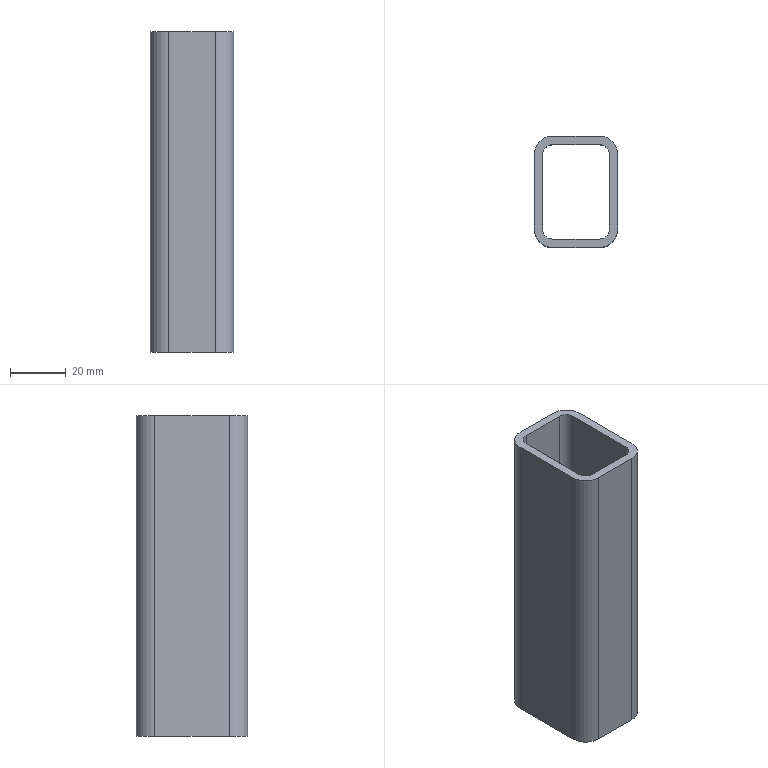Part | STEP file | DIN EN 10305-5 40 x 30 x 3 1785420075848 | 1 solid | 18 faces | box 30 x 40 x 115 mm | volume 41139 mm3 | plane 10 | cylinder 8 | commonest cylinder face diameters 7.2 x4 13.2 x4
STEP:
#1=CARTESIAN_POINT('',(-8.4,-17.,115.));
#2=VERTEX_POINT('',#1);
#3=CARTESIAN_POINT('',(8.4,-17.,115.));
#4=VERTEX_POINT('',#3);
#5=CARTESIAN_POINT('',(4.2,-17.,115.));
#6=DIRECTION('',(1.,0.,0.));
#7=VECTOR('',#6,10.);
#8=LINE('',#5,#7);
#9=EDGE_CURVE('',#2,#4,#8,.T.);
#10=ORIENTED_EDGE('',*,*,#9,.T.);
#11=CARTESIAN_POINT('',(8.4,-17.,0.));
#12=VERTEX_POINT('',#11);
#13=CARTESIAN_POINT('',(8.4,-17.,0.));
#14=DIRECTION('',(0.,0.,1.));
#15=VECTOR('',#14,10.);
#16=LINE('',#13,#15);
#17=EDGE_CURVE('',#12,#4,#16,.T.);
#18=ORIENTED_EDGE('',*,*,#17,.F.);
#19=CARTESIAN_POINT('',(-8.4,-17.,0.));
#20=VERTEX_POINT('',#19);
#21=CARTESIAN_POINT('',(4.2,-17.,0.));
#22=DIRECTION('',(1.,0.,0.));
#23=VECTOR('',#22,10.);
#24=LINE('',#21,#23);
#25=EDGE_CURVE('',#20,#12,#24,.T.);
#26=ORIENTED_EDGE('',*,*,#25,.F.);
#27=CARTESIAN_POINT('',(-8.4,-17.,0.));
#28=DIRECTION('',(0.,0.,1.));
#29=VECTOR('',#28,10.);
#30=LINE('',#27,#29);
#31=EDGE_CURVE('',#20,#2,#30,.T.);
#32=ORIENTED_EDGE('',*,*,#31,.T.);
#33=EDGE_LOOP('',(#10,#18,#26,#32));
#34=FACE_OUTER_BOUND('',#33,.T.);
#35=CARTESIAN_POINT('',(8.4,-17.,0.));
#36=DIRECTION('',(0.,-1.,0.));
#37=DIRECTION('',(0.,0.,-1.));
#38=AXIS2_PLACEMENT_3D('',#35,#36,#37);
#39=PLANE('',#38);
#40=ADVANCED_FACE('',(#34),#39,.F.);
#41=CARTESIAN_POINT('',(12.,-13.4,115.));
#42=VERTEX_POINT('',#41);
#43=CARTESIAN_POINT('',(8.4,-13.4,115.));
#44=DIRECTION('',(0.,0.,1.));
#45=DIRECTION('',(0.,1.,0.));
#46=AXIS2_PLACEMENT_3D('',#43,#44,#45);
#47=CIRCLE('',#46,3.6);
#48=EDGE_CURVE('',#4,#42,#47,.T.);
#49=ORIENTED_EDGE('',*,*,#48,.T.);
#50=CARTESIAN_POINT('',(12.,-13.4,0.));
#51=VERTEX_POINT('',#50);
#52=CARTESIAN_POINT('',(12.,-13.4,0.));
#53=DIRECTION('',(0.,0.,1.));
#54=VECTOR('',#53,10.);
#55=LINE('',#52,#54);
#56=EDGE_CURVE('',#51,#42,#55,.T.);
#57=ORIENTED_EDGE('',*,*,#56,.F.);
#58=CARTESIAN_POINT('',(8.4,-13.4,0.));
#59=DIRECTION('',(0.,0.,1.));
#60=DIRECTION('',(0.,1.,0.));
#61=AXIS2_PLACEMENT_3D('',#58,#59,#60);
#62=CIRCLE('',#61,3.6);
#63=EDGE_CURVE('',#12,#51,#62,.T.);
#64=ORIENTED_EDGE('',*,*,#63,.F.);
#65=ORIENTED_EDGE('',*,*,#17,.T.);
#66=EDGE_LOOP('',(#49,#57,#64,#65));
#67=FACE_OUTER_BOUND('',#66,.T.);
#68=CARTESIAN_POINT('',(8.4,-13.4,0.));
#69=DIRECTION('',(0.,0.,1.));
#70=DIRECTION('',(0.,1.,0.));
#71=AXIS2_PLACEMENT_3D('',#68,#69,#70);
#72=CYLINDRICAL_SURFACE('',#71,3.6);
#73=ADVANCED_FACE('',(#67),#72,.F.);
#74=CARTESIAN_POINT('',(12.,13.4,115.));
#75=VERTEX_POINT('',#74);
#76=CARTESIAN_POINT('',(12.,6.7,115.));
#77=DIRECTION('',(0.,1.,0.));
#78=VECTOR('',#77,10.);
#79=LINE('',#76,#78);
#80=EDGE_CURVE('',#42,#75,#79,.T.);
#81=ORIENTED_EDGE('',*,*,#80,.T.);
#82=CARTESIAN_POINT('',(12.,13.4,0.));
#83=VERTEX_POINT('',#82);
#84=CARTESIAN_POINT('',(12.,13.4,0.));
#85=DIRECTION('',(0.,0.,1.));
#86=VECTOR('',#85,10.);
#87=LINE('',#84,#86);
#88=EDGE_CURVE('',#83,#75,#87,.T.);
#89=ORIENTED_EDGE('',*,*,#88,.F.);
#90=CARTESIAN_POINT('',(12.,6.7,0.));
#91=DIRECTION('',(0.,1.,0.));
#92=VECTOR('',#91,10.);
#93=LINE('',#90,#92);
#94=EDGE_CURVE('',#51,#83,#93,.T.);
#95=ORIENTED_EDGE('',*,*,#94,.F.);
#96=ORIENTED_EDGE('',*,*,#56,.T.);
#97=EDGE_LOOP('',(#81,#89,#95,#96));
#98=FACE_OUTER_BOUND('',#97,.T.);
#99=CARTESIAN_POINT('',(12.,13.4,0.));
#100=DIRECTION('',(1.,0.,0.));
#101=DIRECTION('',(0.,0.,-1.));
#102=AXIS2_PLACEMENT_3D('',#99,#100,#101);
#103=PLANE('',#102);
#104=ADVANCED_FACE('',(#98),#103,.F.);
#105=CARTESIAN_POINT('',(8.4,17.,115.));
#106=VERTEX_POINT('',#105);
#107=CARTESIAN_POINT('',(8.4,13.4,115.));
#108=DIRECTION('',(0.,0.,1.));
#109=DIRECTION('',(-1.,0.,0.));
#110=AXIS2_PLACEMENT_3D('',#107,#108,#109);
#111=CIRCLE('',#110,3.6);
#112=EDGE_CURVE('',#75,#106,#111,.T.);
#113=ORIENTED_EDGE('',*,*,#112,.T.);
#114=CARTESIAN_POINT('',(8.4,17.,0.));
#115=VERTEX_POINT('',#114);
#116=CARTESIAN_POINT('',(8.4,17.,0.));
#117=DIRECTION('',(0.,0.,1.));
#118=VECTOR('',#117,10.);
#119=LINE('',#116,#118);
#120=EDGE_CURVE('',#115,#106,#119,.T.);
#121=ORIENTED_EDGE('',*,*,#120,.F.);
#122=CARTESIAN_POINT('',(8.4,13.4,0.));
#123=DIRECTION('',(0.,0.,1.));
#124=DIRECTION('',(-1.,0.,0.));
#125=AXIS2_PLACEMENT_3D('',#122,#123,#124);
#126=CIRCLE('',#125,3.6);
#127=EDGE_CURVE('',#83,#115,#126,.T.);
#128=ORIENTED_EDGE('',*,*,#127,.F.);
#129=ORIENTED_EDGE('',*,*,#88,.T.);
#130=EDGE_LOOP('',(#113,#121,#128,#129));
#131=FACE_OUTER_BOUND('',#130,.T.);
#132=CARTESIAN_POINT('',(8.4,13.4,0.));
#133=DIRECTION('',(0.,0.,1.));
#134=DIRECTION('',(-1.,0.,0.));
#135=AXIS2_PLACEMENT_3D('',#132,#133,#134);
#136=CYLINDRICAL_SURFACE('',#135,3.6);
#137=ADVANCED_FACE('',(#131),#136,.F.);
#138=CARTESIAN_POINT('',(15.,13.4,115.));
#139=VERTEX_POINT('',#138);
#140=CARTESIAN_POINT('',(15.,-13.4,115.));
#141=VERTEX_POINT('',#140);
#142=CARTESIAN_POINT('',(15.,6.7,115.));
#143=DIRECTION('',(0.,-1.,0.));
#144=VECTOR('',#143,10.);
#145=LINE('',#142,#144);
#146=EDGE_CURVE('',#139,#141,#145,.T.);
#147=ORIENTED_EDGE('',*,*,#146,.T.);
#148=CARTESIAN_POINT('',(15.,-13.4,0.));
#149=VERTEX_POINT('',#148);
#150=CARTESIAN_POINT('',(15.,-13.4,0.));
#151=DIRECTION('',(0.,0.,1.));
#152=VECTOR('',#151,10.);
#153=LINE('',#150,#152);
#154=EDGE_CURVE('',#149,#141,#153,.T.);
#155=ORIENTED_EDGE('',*,*,#154,.F.);
#156=CARTESIAN_POINT('',(15.,13.4,0.));
#157=VERTEX_POINT('',#156);
#158=CARTESIAN_POINT('',(15.,6.7,0.));
#159=DIRECTION('',(0.,-1.,0.));
#160=VECTOR('',#159,10.);
#161=LINE('',#158,#160);
#162=EDGE_CURVE('',#157,#149,#161,.T.);
#163=ORIENTED_EDGE('',*,*,#162,.F.);
#164=CARTESIAN_POINT('',(15.,13.4,0.));
#165=DIRECTION('',(0.,0.,1.));
#166=VECTOR('',#165,10.);
#167=LINE('',#164,#166);
#168=EDGE_CURVE('',#157,#139,#167,.T.);
#169=ORIENTED_EDGE('',*,*,#168,.T.);
#170=EDGE_LOOP('',(#147,#155,#163,#169));
#171=FACE_OUTER_BOUND('',#170,.T.);
#172=CARTESIAN_POINT('',(15.,13.4,0.));
#173=DIRECTION('',(1.,0.,0.));
#174=DIRECTION('',(0.,0.,-1.));
#175=AXIS2_PLACEMENT_3D('',#172,#173,#174);
#176=PLANE('',#175);
#177=ADVANCED_FACE('',(#171),#176,.T.);
#178=CARTESIAN_POINT('',(8.4,-20.,115.));
#179=VERTEX_POINT('',#178);
#180=CARTESIAN_POINT('',(8.4,-13.4,115.));
#181=DIRECTION('',(0.,0.,-1.));
#182=DIRECTION('',(0.,1.,0.));
#183=AXIS2_PLACEMENT_3D('',#180,#181,#182);
#184=CIRCLE('',#183,6.6);
#185=EDGE_CURVE('',#141,#179,#184,.T.);
#186=ORIENTED_EDGE('',*,*,#185,.T.);
#187=CARTESIAN_POINT('',(8.4,-20.,0.));
#188=VERTEX_POINT('',#187);
#189=CARTESIAN_POINT('',(8.4,-20.,0.));
#190=DIRECTION('',(0.,0.,1.));
#191=VECTOR('',#190,10.);
#192=LINE('',#189,#191);
#193=EDGE_CURVE('',#188,#179,#192,.T.);
#194=ORIENTED_EDGE('',*,*,#193,.F.);
#195=CARTESIAN_POINT('',(8.4,-13.4,0.));
#196=DIRECTION('',(0.,0.,-1.));
#197=DIRECTION('',(0.,1.,0.));
#198=AXIS2_PLACEMENT_3D('',#195,#196,#197);
#199=CIRCLE('',#198,6.6);
#200=EDGE_CURVE('',#149,#188,#199,.T.);
#201=ORIENTED_EDGE('',*,*,#200,.F.);
#202=ORIENTED_EDGE('',*,*,#154,.T.);
#203=EDGE_LOOP('',(#186,#194,#201,#202));
#204=FACE_OUTER_BOUND('',#203,.T.);
#205=CARTESIAN_POINT('',(8.4,-13.4,0.));
#206=DIRECTION('',(0.,0.,1.));
#207=DIRECTION('',(0.,1.,0.));
#208=AXIS2_PLACEMENT_3D('',#205,#206,#207);
#209=CYLINDRICAL_SURFACE('',#208,6.6);
#210=ADVANCED_FACE('',(#204),#209,.T.);
#211=CARTESIAN_POINT('',(-8.4,-20.,115.));
#212=VERTEX_POINT('',#211);
#213=CARTESIAN_POINT('',(4.2,-20.,115.));
#214=DIRECTION('',(-1.,0.,0.));
#215=VECTOR('',#214,10.);
#216=LINE('',#213,#215);
#217=EDGE_CURVE('',#179,#212,#216,.T.);
#218=ORIENTED_EDGE('',*,*,#217,.T.);
#219=CARTESIAN_POINT('',(-8.4,-20.,0.));
#220=VERTEX_POINT('',#219);
#221=CARTESIAN_POINT('',(-8.4,-20.,0.));
#222=DIRECTION('',(0.,0.,1.));
#223=VECTOR('',#222,10.);
#224=LINE('',#221,#223);
#225=EDGE_CURVE('',#220,#212,#224,.T.);
#226=ORIENTED_EDGE('',*,*,#225,.F.);
#227=CARTESIAN_POINT('',(4.2,-20.,0.));
#228=DIRECTION('',(-1.,0.,0.));
#229=VECTOR('',#228,10.);
#230=LINE('',#227,#229);
#231=EDGE_CURVE('',#188,#220,#230,.T.);
#232=ORIENTED_EDGE('',*,*,#231,.F.);
#233=ORIENTED_EDGE('',*,*,#193,.T.);
#234=EDGE_LOOP('',(#218,#226,#232,#233));
#235=FACE_OUTER_BOUND('',#234,.T.);
#236=CARTESIAN_POINT('',(8.4,-20.,0.));
#237=DIRECTION('',(0.,-1.,0.));
#238=DIRECTION('',(0.,0.,-1.));
#239=AXIS2_PLACEMENT_3D('',#236,#237,#238);
#240=PLANE('',#239);
#241=ADVANCED_FACE('',(#235),#240,.T.);
#242=CARTESIAN_POINT('',(-15.,-13.4,115.));
#243=VERTEX_POINT('',#242);
#244=CARTESIAN_POINT('',(-8.4,-13.4,115.));
#245=DIRECTION('',(0.,0.,-1.));
#246=DIRECTION('',(1.,0.,0.));
#247=AXIS2_PLACEMENT_3D('',#244,#245,#246);
#248=CIRCLE('',#247,6.6);
#249=EDGE_CURVE('',#212,#243,#248,.T.);
#250=ORIENTED_EDGE('',*,*,#249,.T.);
#251=CARTESIAN_POINT('',(-15.,-13.4,0.));
#252=VERTEX_POINT('',#251);
#253=CARTESIAN_POINT('',(-15.,-13.4,0.));
#254=DIRECTION('',(0.,0.,1.));
#255=VECTOR('',#254,10.);
#256=LINE('',#253,#255);
#257=EDGE_CURVE('',#252,#243,#256,.T.);
#258=ORIENTED_EDGE('',*,*,#257,.F.);
#259=CARTESIAN_POINT('',(-8.4,-13.4,0.));
#260=DIRECTION('',(0.,0.,-1.));
#261=DIRECTION('',(1.,0.,0.));
#262=AXIS2_PLACEMENT_3D('',#259,#260,#261);
#263=CIRCLE('',#262,6.6);
#264=EDGE_CURVE('',#220,#252,#263,.T.);
#265=ORIENTED_EDGE('',*,*,#264,.F.);
#266=ORIENTED_EDGE('',*,*,#225,.T.);
#267=EDGE_LOOP('',(#250,#258,#265,#266));
#268=FACE_OUTER_BOUND('',#267,.T.);
#269=CARTESIAN_POINT('',(-8.4,-13.4,0.));
#270=DIRECTION('',(0.,0.,1.));
#271=DIRECTION('',(1.,0.,0.));
#272=AXIS2_PLACEMENT_3D('',#269,#270,#271);
#273=CYLINDRICAL_SURFACE('',#272,6.6);
#274=ADVANCED_FACE('',(#268),#273,.T.);
#275=CARTESIAN_POINT('',(-8.4,17.,115.));
#276=VERTEX_POINT('',#275);
#277=CARTESIAN_POINT('',(-4.2,17.,115.));
#278=DIRECTION('',(-1.,0.,0.));
#279=VECTOR('',#278,10.);
#280=LINE('',#277,#279);
#281=EDGE_CURVE('',#106,#276,#280,.T.);
#282=ORIENTED_EDGE('',*,*,#281,.T.);
#283=CARTESIAN_POINT('',(-8.4,17.,0.));
#284=VERTEX_POINT('',#283);
#285=CARTESIAN_POINT('',(-8.4,17.,0.));
#286=DIRECTION('',(0.,0.,1.));
#287=VECTOR('',#286,10.);
#288=LINE('',#285,#287);
#289=EDGE_CURVE('',#284,#276,#288,.T.);
#290=ORIENTED_EDGE('',*,*,#289,.F.);
#291=CARTESIAN_POINT('',(-4.2,17.,0.));
#292=DIRECTION('',(-1.,0.,0.));
#293=VECTOR('',#292,10.);
#294=LINE('',#291,#293);
#295=EDGE_CURVE('',#115,#284,#294,.T.);
#296=ORIENTED_EDGE('',*,*,#295,.F.);
#297=ORIENTED_EDGE('',*,*,#120,.T.);
#298=EDGE_LOOP('',(#282,#290,#296,#297));
#299=FACE_OUTER_BOUND('',#298,.T.);
#300=CARTESIAN_POINT('',(-8.4,17.,0.));
#301=DIRECTION('',(0.,1.,0.));
#302=DIRECTION('',(0.,0.,1.));
#303=AXIS2_PLACEMENT_3D('',#300,#301,#302);
#304=PLANE('',#303);
#305=ADVANCED_FACE('',(#299),#304,.F.);
#306=CARTESIAN_POINT('',(-12.,-13.4,115.));
#307=VERTEX_POINT('',#306);
#308=CARTESIAN_POINT('',(-8.4,-13.4,115.));
#309=DIRECTION('',(0.,0.,1.));
#310=DIRECTION('',(1.,0.,0.));
#311=AXIS2_PLACEMENT_3D('',#308,#309,#310);
#312=CIRCLE('',#311,3.6);
#313=EDGE_CURVE('',#307,#2,#312,.T.);
#314=ORIENTED_EDGE('',*,*,#313,.T.);
#315=ORIENTED_EDGE('',*,*,#31,.F.);
#316=CARTESIAN_POINT('',(-12.,-13.4,0.));
#317=VERTEX_POINT('',#316);
#318=CARTESIAN_POINT('',(-8.4,-13.4,0.));
#319=DIRECTION('',(0.,0.,1.));
#320=DIRECTION('',(1.,0.,0.));
#321=AXIS2_PLACEMENT_3D('',#318,#319,#320);
#322=CIRCLE('',#321,3.6);
#323=EDGE_CURVE('',#317,#20,#322,.T.);
#324=ORIENTED_EDGE('',*,*,#323,.F.);
#325=CARTESIAN_POINT('',(-12.,-13.4,0.));
#326=DIRECTION('',(0.,0.,1.));
#327=VECTOR('',#326,10.);
#328=LINE('',#325,#327);
#329=EDGE_CURVE('',#317,#307,#328,.T.);
#330=ORIENTED_EDGE('',*,*,#329,.T.);
#331=EDGE_LOOP('',(#314,#315,#324,#330));
#332=FACE_OUTER_BOUND('',#331,.T.);
#333=CARTESIAN_POINT('',(-8.4,-13.4,0.));
#334=DIRECTION('',(0.,0.,1.));
#335=DIRECTION('',(1.,0.,0.));
#336=AXIS2_PLACEMENT_3D('',#333,#334,#335);
#337=CYLINDRICAL_SURFACE('',#336,3.6);
#338=ADVANCED_FACE('',(#332),#337,.F.);
#339=CARTESIAN_POINT('',(-12.,13.4,115.));
#340=VERTEX_POINT('',#339);
#341=CARTESIAN_POINT('',(-12.,-6.7,115.));
#342=DIRECTION('',(0.,-1.,0.));
#343=VECTOR('',#342,10.);
#344=LINE('',#341,#343);
#345=EDGE_CURVE('',#340,#307,#344,.T.);
#346=ORIENTED_EDGE('',*,*,#345,.T.);
#347=ORIENTED_EDGE('',*,*,#329,.F.);
#348=CARTESIAN_POINT('',(-12.,13.4,0.));
#349=VERTEX_POINT('',#348);
#350=CARTESIAN_POINT('',(-12.,-6.7,0.));
#351=DIRECTION('',(0.,-1.,0.));
#352=VECTOR('',#351,10.);
#353=LINE('',#350,#352);
#354=EDGE_CURVE('',#349,#317,#353,.T.);
#355=ORIENTED_EDGE('',*,*,#354,.F.);
#356=CARTESIAN_POINT('',(-12.,13.4,0.));
#357=DIRECTION('',(0.,0.,1.));
#358=VECTOR('',#357,10.);
#359=LINE('',#356,#358);
#360=EDGE_CURVE('',#349,#340,#359,.T.);
#361=ORIENTED_EDGE('',*,*,#360,.T.);
#362=EDGE_LOOP('',(#346,#347,#355,#361));
#363=FACE_OUTER_BOUND('',#362,.T.);
#364=CARTESIAN_POINT('',(-12.,-13.4,0.));
#365=DIRECTION('',(-1.,0.,0.));
#366=DIRECTION('',(0.,0.,1.));
#367=AXIS2_PLACEMENT_3D('',#364,#365,#366);
#368=PLANE('',#367);
#369=ADVANCED_FACE('',(#363),#368,.F.);
#370=CARTESIAN_POINT('',(-8.4,13.4,115.));
#371=DIRECTION('',(0.,0.,1.));
#372=DIRECTION('',(0.,-1.,0.));
#373=AXIS2_PLACEMENT_3D('',#370,#371,#372);
#374=CIRCLE('',#373,3.6);
#375=EDGE_CURVE('',#276,#340,#374,.T.);
#376=ORIENTED_EDGE('',*,*,#375,.T.);
#377=ORIENTED_EDGE('',*,*,#360,.F.);
#378=CARTESIAN_POINT('',(-8.4,13.4,0.));
#379=DIRECTION('',(0.,0.,1.));
#380=DIRECTION('',(0.,-1.,0.));
#381=AXIS2_PLACEMENT_3D('',#378,#379,#380);
#382=CIRCLE('',#381,3.6);
#383=EDGE_CURVE('',#284,#349,#382,.T.);
#384=ORIENTED_EDGE('',*,*,#383,.F.);
#385=ORIENTED_EDGE('',*,*,#289,.T.);
#386=EDGE_LOOP('',(#376,#377,#384,#385));
#387=FACE_OUTER_BOUND('',#386,.T.);
#388=CARTESIAN_POINT('',(-8.4,13.4,0.));
#389=DIRECTION('',(0.,0.,1.));
#390=DIRECTION('',(0.,-1.,0.));
#391=AXIS2_PLACEMENT_3D('',#388,#389,#390);
#392=CYLINDRICAL_SURFACE('',#391,3.6);
#393=ADVANCED_FACE('',(#387),#392,.F.);
#394=CARTESIAN_POINT('',(-15.,13.4,115.));
#395=VERTEX_POINT('',#394);
#396=CARTESIAN_POINT('',(-15.,-6.7,115.));
#397=DIRECTION('',(0.,1.,0.));
#398=VECTOR('',#397,10.);
#399=LINE('',#396,#398);
#400=EDGE_CURVE('',#243,#395,#399,.T.);
#401=ORIENTED_EDGE('',*,*,#400,.T.);
#402=CARTESIAN_POINT('',(-15.,13.4,0.));
#403=VERTEX_POINT('',#402);
#404=CARTESIAN_POINT('',(-15.,13.4,0.));
#405=DIRECTION('',(0.,0.,1.));
#406=VECTOR('',#405,10.);
#407=LINE('',#404,#406);
#408=EDGE_CURVE('',#403,#395,#407,.T.);
#409=ORIENTED_EDGE('',*,*,#408,.F.);
#410=CARTESIAN_POINT('',(-15.,-6.7,0.));
#411=DIRECTION('',(0.,1.,0.));
#412=VECTOR('',#411,10.);
#413=LINE('',#410,#412);
#414=EDGE_CURVE('',#252,#403,#413,.T.);
#415=ORIENTED_EDGE('',*,*,#414,.F.);
#416=ORIENTED_EDGE('',*,*,#257,.T.);
#417=EDGE_LOOP('',(#401,#409,#415,#416));
#418=FACE_OUTER_BOUND('',#417,.T.);
#419=CARTESIAN_POINT('',(-15.,-13.4,0.));
#420=DIRECTION('',(-1.,0.,0.));
#421=DIRECTION('',(0.,0.,1.));
#422=AXIS2_PLACEMENT_3D('',#419,#420,#421);
#423=PLANE('',#422);
#424=ADVANCED_FACE('',(#418),#423,.T.);
#425=CARTESIAN_POINT('',(-8.4,20.,115.));
#426=VERTEX_POINT('',#425);
#427=CARTESIAN_POINT('',(-8.4,13.4,115.));
#428=DIRECTION('',(0.,0.,-1.));
#429=DIRECTION('',(0.,-1.,0.));
#430=AXIS2_PLACEMENT_3D('',#427,#428,#429);
#431=CIRCLE('',#430,6.6);
#432=EDGE_CURVE('',#395,#426,#431,.T.);
#433=ORIENTED_EDGE('',*,*,#432,.T.);
#434=CARTESIAN_POINT('',(-8.4,20.,0.));
#435=VERTEX_POINT('',#434);
#436=CARTESIAN_POINT('',(-8.4,20.,0.));
#437=DIRECTION('',(0.,0.,1.));
#438=VECTOR('',#437,10.);
#439=LINE('',#436,#438);
#440=EDGE_CURVE('',#435,#426,#439,.T.);
#441=ORIENTED_EDGE('',*,*,#440,.F.);
#442=CARTESIAN_POINT('',(-8.4,13.4,0.));
#443=DIRECTION('',(0.,0.,-1.));
#444=DIRECTION('',(0.,-1.,0.));
#445=AXIS2_PLACEMENT_3D('',#442,#443,#444);
#446=CIRCLE('',#445,6.6);
#447=EDGE_CURVE('',#403,#435,#446,.T.);
#448=ORIENTED_EDGE('',*,*,#447,.F.);
#449=ORIENTED_EDGE('',*,*,#408,.T.);
#450=EDGE_LOOP('',(#433,#441,#448,#449));
#451=FACE_OUTER_BOUND('',#450,.T.);
#452=CARTESIAN_POINT('',(-8.4,13.4,0.));
#453=DIRECTION('',(0.,0.,1.));
#454=DIRECTION('',(0.,-1.,0.));
#455=AXIS2_PLACEMENT_3D('',#452,#453,#454);
#456=CYLINDRICAL_SURFACE('',#455,6.6);
#457=ADVANCED_FACE('',(#451),#456,.T.);
#458=CARTESIAN_POINT('',(8.4,20.,115.));
#459=VERTEX_POINT('',#458);
#460=CARTESIAN_POINT('',(-4.2,20.,115.));
#461=DIRECTION('',(1.,0.,0.));
#462=VECTOR('',#461,10.);
#463=LINE('',#460,#462);
#464=EDGE_CURVE('',#426,#459,#463,.T.);
#465=ORIENTED_EDGE('',*,*,#464,.T.);
#466=CARTESIAN_POINT('',(8.4,20.,0.));
#467=VERTEX_POINT('',#466);
#468=CARTESIAN_POINT('',(8.4,20.,0.));
#469=DIRECTION('',(0.,0.,1.));
#470=VECTOR('',#469,10.);
#471=LINE('',#468,#470);
#472=EDGE_CURVE('',#467,#459,#471,.T.);
#473=ORIENTED_EDGE('',*,*,#472,.F.);
#474=CARTESIAN_POINT('',(-4.2,20.,0.));
#475=DIRECTION('',(1.,0.,0.));
#476=VECTOR('',#475,10.);
#477=LINE('',#474,#476);
#478=EDGE_CURVE('',#435,#467,#477,.T.);
#479=ORIENTED_EDGE('',*,*,#478,.F.);
#480=ORIENTED_EDGE('',*,*,#440,.T.);
#481=EDGE_LOOP('',(#465,#473,#479,#480));
#482=FACE_OUTER_BOUND('',#481,.T.);
#483=CARTESIAN_POINT('',(-8.4,20.,0.));
#484=DIRECTION('',(0.,1.,0.));
#485=DIRECTION('',(0.,0.,1.));
#486=AXIS2_PLACEMENT_3D('',#483,#484,#485);
#487=PLANE('',#486);
#488=ADVANCED_FACE('',(#482),#487,.T.);
#489=CARTESIAN_POINT('',(8.4,13.4,115.));
#490=DIRECTION('',(0.,0.,-1.));
#491=DIRECTION('',(-1.,0.,0.));
#492=AXIS2_PLACEMENT_3D('',#489,#490,#491);
#493=CIRCLE('',#492,6.6);
#494=EDGE_CURVE('',#459,#139,#493,.T.);
#495=ORIENTED_EDGE('',*,*,#494,.T.);
#496=ORIENTED_EDGE('',*,*,#168,.F.);
#497=CARTESIAN_POINT('',(8.4,13.4,0.));
#498=DIRECTION('',(0.,0.,-1.));
#499=DIRECTION('',(-1.,0.,0.));
#500=AXIS2_PLACEMENT_3D('',#497,#498,#499);
#501=CIRCLE('',#500,6.6);
#502=EDGE_CURVE('',#467,#157,#501,.T.);
#503=ORIENTED_EDGE('',*,*,#502,.F.);
#504=ORIENTED_EDGE('',*,*,#472,.T.);
#505=EDGE_LOOP('',(#495,#496,#503,#504));
#506=FACE_OUTER_BOUND('',#505,.T.);
#507=CARTESIAN_POINT('',(8.4,13.4,0.));
#508=DIRECTION('',(0.,0.,1.));
#509=DIRECTION('',(-1.,0.,0.));
#510=AXIS2_PLACEMENT_3D('',#507,#508,#509);
#511=CYLINDRICAL_SURFACE('',#510,6.6);
#512=ADVANCED_FACE('',(#506),#511,.T.);
#513=ORIENTED_EDGE('',*,*,#414,.T.);
#514=ORIENTED_EDGE('',*,*,#447,.T.);
#515=ORIENTED_EDGE('',*,*,#478,.T.);
#516=ORIENTED_EDGE('',*,*,#502,.T.);
#517=ORIENTED_EDGE('',*,*,#162,.T.);
#518=ORIENTED_EDGE('',*,*,#200,.T.);
#519=ORIENTED_EDGE('',*,*,#231,.T.);
#520=ORIENTED_EDGE('',*,*,#264,.T.);
#521=EDGE_LOOP('',(#513,#514,#515,#516,#517,#518,#519,#520));
#522=FACE_OUTER_BOUND('',#521,.T.);
#523=ORIENTED_EDGE('',*,*,#295,.T.);
#524=ORIENTED_EDGE('',*,*,#383,.T.);
#525=ORIENTED_EDGE('',*,*,#354,.T.);
#526=ORIENTED_EDGE('',*,*,#323,.T.);
#527=ORIENTED_EDGE('',*,*,#25,.T.);
#528=ORIENTED_EDGE('',*,*,#63,.T.);
#529=ORIENTED_EDGE('',*,*,#94,.T.);
#530=ORIENTED_EDGE('',*,*,#127,.T.);
#531=EDGE_LOOP('',(#523,#524,#525,#526,#527,#528,#529,#530));
#532=FACE_BOUND('',#531,.T.);
#533=CARTESIAN_POINT('',(0.,0.,0.));
#534=DIRECTION('',(0.,0.,1.));
#535=DIRECTION('',(1.,0.,0.));
#536=AXIS2_PLACEMENT_3D('',#533,#534,#535);
#537=PLANE('',#536);
#538=ADVANCED_FACE('',(#522,#532),#537,.F.);
#539=ORIENTED_EDGE('',*,*,#400,.F.);
#540=ORIENTED_EDGE('',*,*,#249,.F.);
#541=ORIENTED_EDGE('',*,*,#217,.F.);
#542=ORIENTED_EDGE('',*,*,#185,.F.);
#543=ORIENTED_EDGE('',*,*,#146,.F.);
#544=ORIENTED_EDGE('',*,*,#494,.F.);
#545=ORIENTED_EDGE('',*,*,#464,.F.);
#546=ORIENTED_EDGE('',*,*,#432,.F.);
#547=EDGE_LOOP('',(#539,#540,#541,#542,#543,#544,#545,#546));
#548=FACE_OUTER_BOUND('',#547,.T.);
#549=ORIENTED_EDGE('',*,*,#281,.F.);
#550=ORIENTED_EDGE('',*,*,#112,.F.);
#551=ORIENTED_EDGE('',*,*,#80,.F.);
#552=ORIENTED_EDGE('',*,*,#48,.F.);
#553=ORIENTED_EDGE('',*,*,#9,.F.);
#554=ORIENTED_EDGE('',*,*,#313,.F.);
#555=ORIENTED_EDGE('',*,*,#345,.F.);
#556=ORIENTED_EDGE('',*,*,#375,.F.);
#557=EDGE_LOOP('',(#549,#550,#551,#552,#553,#554,#555,#556));
#558=FACE_BOUND('',#557,.T.);
#559=CARTESIAN_POINT('',(0.,0.,115.));
#560=DIRECTION('',(0.,0.,1.));
#561=DIRECTION('',(1.,0.,0.));
#562=AXIS2_PLACEMENT_3D('',#559,#560,#561);
#563=PLANE('',#562);
#564=ADVANCED_FACE('',(#548,#558),#563,.T.);
#565=CLOSED_SHELL('',(#40,#73,#104,#137,#177,#210,#241,#274,#305,#338,#369,#393,#424,#457,#488,#512,#538,#564));
#566=MANIFOLD_SOLID_BREP('',#565);
#567=(LENGTH_UNIT()NAMED_UNIT(*)SI_UNIT(.MILLI.,.METRE.));
#568=UNCERTAINTY_MEASURE_WITH_UNIT(LENGTH_MEASURE(0.01),#567,'','');
#569=(NAMED_UNIT(*)PLANE_ANGLE_UNIT()SI_UNIT($,.RADIAN.));
#570=(NAMED_UNIT(*)SI_UNIT($,.STERADIAN.)SOLID_ANGLE_UNIT());
#571=(GEOMETRIC_REPRESENTATION_CONTEXT(3)GLOBAL_UNCERTAINTY_ASSIGNED_CONTEXT((#568))GLOBAL_UNIT_ASSIGNED_CONTEXT((#567,#569,#570))REPRESENTATION_CONTEXT('',''));
#572=ADVANCED_BREP_SHAPE_REPRESENTATION('',(#566),#571);